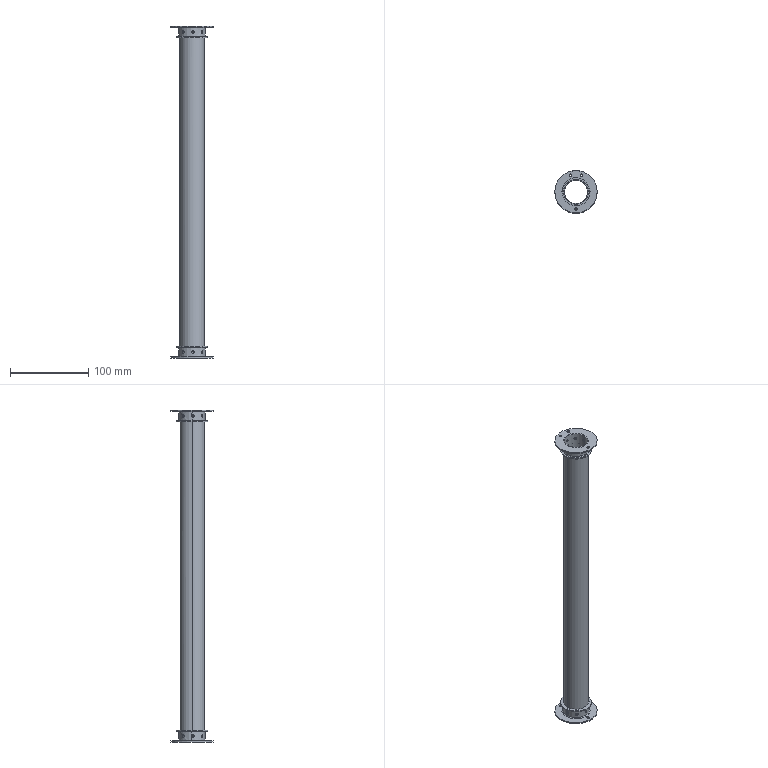Part | SolidWorks | features BaseBody 3 | 3 solids | 98 faces | box 54 x 54 x 423.4 mm | volume 44440 mm3 | cylinder 50 | spline 38 | plane 10 | commonest cylinder face diameters 3.2 x30 31.75 x6 33.782 x4 40 x4 54 x4 29.972 x2